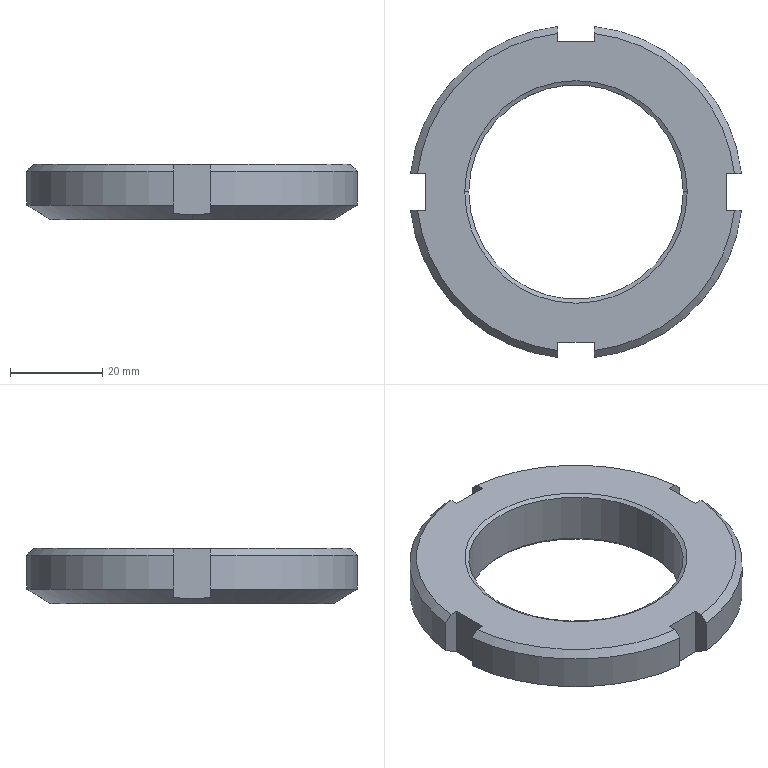Part | SolidWorks | features BaseBody 1 | 1 solid | 30 faces | box 71.554 x 71.554 x 12 mm | volume 25355 mm3 | plane 14 | cone 10 | cylinder 6 | commonest cylinder face diameters 72 x4 46.376 x2
STEP:
#1=CARTESIAN_POINT('',(-23.188,0.,-0.5));
#2=VERTEX_POINT('',#1);
#3=CARTESIAN_POINT('',(23.188,0.,-0.5));
#4=VERTEX_POINT('',#3);
#5=CARTESIAN_POINT('',(0.,0.,-0.5));
#6=DIRECTION('',(0.,0.,1.));
#7=DIRECTION('',(1.,0.,0.));
#8=AXIS2_PLACEMENT_3D('',#5,#6,#7);
#9=CIRCLE('',#8,23.188);
#10=EDGE_CURVE('',#2,#4,#9,.T.);
#11=ORIENTED_EDGE('',*,*,#10,.F.);
#12=CARTESIAN_POINT('',(-24.054,0.,0.));
#13=VERTEX_POINT('',#12);
#14=CARTESIAN_POINT('',(-24.054,0.,0.));
#15=DIRECTION('',(-0.866,0.,0.5));
#16=VECTOR('',#15,1000.);
#17=LINE('',#14,#16);
#18=EDGE_CURVE('',#2,#13,#17,.T.);
#19=ORIENTED_EDGE('',*,*,#18,.T.);
#20=CARTESIAN_POINT('',(24.054,0.,0.));
#21=VERTEX_POINT('',#20);
#22=CARTESIAN_POINT('',(0.,0.,0.));
#23=DIRECTION('',(0.,0.,-1.));
#24=DIRECTION('',(1.,0.,0.));
#25=AXIS2_PLACEMENT_3D('',#22,#23,#24);
#26=CIRCLE('',#25,24.054);
#27=EDGE_CURVE('',#21,#13,#26,.T.);
#28=ORIENTED_EDGE('',*,*,#27,.F.);
#29=CARTESIAN_POINT('',(24.054,0.,0.));
#30=DIRECTION('',(0.866,0.,0.5));
#31=VECTOR('',#30,1000.);
#32=LINE('',#29,#31);
#33=EDGE_CURVE('',#4,#21,#32,.T.);
#34=ORIENTED_EDGE('',*,*,#33,.F.);
#35=EDGE_LOOP('',(#11,#19,#28,#34));
#36=FACE_OUTER_BOUND('',#35,.T.);
#37=CARTESIAN_POINT('',(0.,0.,0.));
#38=DIRECTION('',(0.,0.,1.));
#39=DIRECTION('',(1.,0.,0.));
#40=AXIS2_PLACEMENT_3D('',#37,#38,#39);
#41=CONICAL_SURFACE('',#40,24.054,1.047);
#42=ADVANCED_FACE('',(#36),#41,.F.);
#43=CARTESIAN_POINT('',(-23.188,0.,-11.3));
#44=VERTEX_POINT('',#43);
#45=CARTESIAN_POINT('',(23.188,0.,-11.3));
#46=VERTEX_POINT('',#45);
#47=CARTESIAN_POINT('',(0.,0.,-11.3));
#48=DIRECTION('',(0.,0.,1.));
#49=DIRECTION('',(1.,0.,0.));
#50=AXIS2_PLACEMENT_3D('',#47,#48,#49);
#51=CIRCLE('',#50,23.188);
#52=EDGE_CURVE('',#44,#46,#51,.T.);
#53=ORIENTED_EDGE('',*,*,#52,.F.);
#54=CARTESIAN_POINT('',(-23.188,0.,-12.));
#55=DIRECTION('',(0.,0.,1.));
#56=VECTOR('',#55,1000.);
#57=LINE('',#54,#56);
#58=EDGE_CURVE('',#44,#2,#57,.T.);
#59=ORIENTED_EDGE('',*,*,#58,.T.);
#60=ORIENTED_EDGE('',*,*,#10,.T.);
#61=CARTESIAN_POINT('',(23.188,0.,-12.));
#62=DIRECTION('',(0.,0.,1.));
#63=VECTOR('',#62,1000.);
#64=LINE('',#61,#63);
#65=EDGE_CURVE('',#46,#4,#64,.T.);
#66=ORIENTED_EDGE('',*,*,#65,.F.);
#67=EDGE_LOOP('',(#53,#59,#60,#66));
#68=FACE_OUTER_BOUND('',#67,.T.);
#69=CARTESIAN_POINT('',(0.,0.,-12.));
#70=DIRECTION('',(0.,0.,1.));
#71=DIRECTION('',(1.,0.,0.));
#72=AXIS2_PLACEMENT_3D('',#69,#70,#71);
#73=CYLINDRICAL_SURFACE('',#72,23.188);
#74=ADVANCED_FACE('',(#68),#73,.F.);
#75=CARTESIAN_POINT('',(0.,-30.5,-12.));
#76=VERTEX_POINT('',#75);
#77=CARTESIAN_POINT('',(0.,30.5,-12.));
#78=VERTEX_POINT('',#77);
#79=CARTESIAN_POINT('',(0.,0.,-12.));
#80=DIRECTION('',(0.,0.,1.));
#81=DIRECTION('',(0.,-1.,0.));
#82=AXIS2_PLACEMENT_3D('',#79,#80,#81);
#83=CIRCLE('',#82,30.5);
#84=EDGE_CURVE('',#76,#78,#83,.T.);
#85=ORIENTED_EDGE('',*,*,#84,.T.);
#86=CARTESIAN_POINT('',(0.,32.5,-10.845));
#87=VERTEX_POINT('',#86);
#88=CARTESIAN_POINT('',(0.,36.,-8.825));
#89=DIRECTION('',(0.,0.866,0.5));
#90=VECTOR('',#89,1000.);
#91=LINE('',#88,#90);
#92=EDGE_CURVE('',#78,#87,#91,.T.);
#93=ORIENTED_EDGE('',*,*,#92,.T.);
#94=CARTESIAN_POINT('',(4.,32.5,-10.704));
#95=VERTEX_POINT('',#94);
#96=CARTESIAN_POINT('',(0.,32.5,-10.845));
#97=CARTESIAN_POINT('',(1.333,32.5,-10.845));
#98=CARTESIAN_POINT('',(2.667,32.5,-10.798));
#99=CARTESIAN_POINT('',(4.,32.5,-10.704));
#100=B_SPLINE_CURVE_WITH_KNOTS('',3,(#96,#97,#98,#99),.UNSPECIFIED.,.F.,.F.,(4,4),(0.004,0.008),.UNSPECIFIED.);
#101=EDGE_CURVE('',#87,#95,#100,.T.);
#102=ORIENTED_EDGE('',*,*,#101,.T.);
#103=CARTESIAN_POINT('',(4.,35.777,-8.825));
#104=VERTEX_POINT('',#103);
#105=CARTESIAN_POINT('',(4.,32.5,-10.704));
#106=CARTESIAN_POINT('',(4.,33.593,-10.078));
#107=CARTESIAN_POINT('',(4.,34.685,-9.451));
#108=CARTESIAN_POINT('',(4.,35.777,-8.825));
#109=B_SPLINE_CURVE_WITH_KNOTS('',3,(#105,#106,#107,#108),.UNSPECIFIED.,.F.,.F.,(4,4),(0.,0.003778),.UNSPECIFIED.);
#110=EDGE_CURVE('',#95,#104,#109,.T.);
#111=ORIENTED_EDGE('',*,*,#110,.T.);
#112=CARTESIAN_POINT('',(35.777,4.,-8.825));
#113=VERTEX_POINT('',#112);
#114=CARTESIAN_POINT('',(0.,0.,-8.825));
#115=DIRECTION('',(0.,0.,-1.));
#116=DIRECTION('',(1.,0.,0.));
#117=AXIS2_PLACEMENT_3D('',#114,#115,#116);
#118=CIRCLE('',#117,36.);
#119=EDGE_CURVE('',#104,#113,#118,.T.);
#120=ORIENTED_EDGE('',*,*,#119,.T.);
#121=CARTESIAN_POINT('',(32.5,4.,-10.704));
#122=VERTEX_POINT('',#121);
#123=CARTESIAN_POINT('',(35.777,4.,-8.825));
#124=CARTESIAN_POINT('',(34.685,4.,-9.451));
#125=CARTESIAN_POINT('',(33.593,4.,-10.078));
#126=CARTESIAN_POINT('',(32.5,4.,-10.704));
#127=B_SPLINE_CURVE_WITH_KNOTS('',3,(#123,#124,#125,#126),.UNSPECIFIED.,.F.,.F.,(4,4),(0.,0.003778),.UNSPECIFIED.);
#128=EDGE_CURVE('',#113,#122,#127,.T.);
#129=ORIENTED_EDGE('',*,*,#128,.T.);
#130=CARTESIAN_POINT('',(32.5,-4.,-10.704));
#131=VERTEX_POINT('',#130);
#132=CARTESIAN_POINT('',(32.5,4.,-10.704));
#133=CARTESIAN_POINT('',(32.5,1.337,-10.892));
#134=CARTESIAN_POINT('',(32.5,-1.337,-10.892));
#135=CARTESIAN_POINT('',(32.5,-4.,-10.704));
#136=B_SPLINE_CURVE_WITH_KNOTS('',3,(#132,#133,#134,#135),.UNSPECIFIED.,.F.,.F.,(4,4),(-0.004003,0.004003),.UNSPECIFIED.);
#137=EDGE_CURVE('',#122,#131,#136,.T.);
#138=ORIENTED_EDGE('',*,*,#137,.T.);
#139=CARTESIAN_POINT('',(35.777,-4.,-8.825));
#140=VERTEX_POINT('',#139);
#141=CARTESIAN_POINT('',(32.5,-4.,-10.704));
#142=CARTESIAN_POINT('',(33.593,-4.,-10.078));
#143=CARTESIAN_POINT('',(34.685,-4.,-9.451));
#144=CARTESIAN_POINT('',(35.777,-4.,-8.825));
#145=B_SPLINE_CURVE_WITH_KNOTS('',3,(#141,#142,#143,#144),.UNSPECIFIED.,.F.,.F.,(4,4),(0.,0.003778),.UNSPECIFIED.);
#146=EDGE_CURVE('',#131,#140,#145,.T.);
#147=ORIENTED_EDGE('',*,*,#146,.T.);
#148=CARTESIAN_POINT('',(4.,-35.777,-8.825));
#149=VERTEX_POINT('',#148);
#150=CARTESIAN_POINT('',(0.,0.,-8.825));
#151=DIRECTION('',(0.,0.,-1.));
#152=DIRECTION('',(1.,0.,0.));
#153=AXIS2_PLACEMENT_3D('',#150,#151,#152);
#154=CIRCLE('',#153,36.);
#155=EDGE_CURVE('',#140,#149,#154,.T.);
#156=ORIENTED_EDGE('',*,*,#155,.T.);
#157=CARTESIAN_POINT('',(4.,-32.5,-10.704));
#158=VERTEX_POINT('',#157);
#159=CARTESIAN_POINT('',(4.,-35.777,-8.825));
#160=CARTESIAN_POINT('',(4.,-34.685,-9.451));
#161=CARTESIAN_POINT('',(4.,-33.593,-10.078));
#162=CARTESIAN_POINT('',(4.,-32.5,-10.704));
#163=B_SPLINE_CURVE_WITH_KNOTS('',3,(#159,#160,#161,#162),.UNSPECIFIED.,.F.,.F.,(4,4),(0.,0.003778),.UNSPECIFIED.);
#164=EDGE_CURVE('',#149,#158,#163,.T.);
#165=ORIENTED_EDGE('',*,*,#164,.T.);
#166=CARTESIAN_POINT('',(0.,-32.5,-10.845));
#167=VERTEX_POINT('',#166);
#168=CARTESIAN_POINT('',(4.,-32.5,-10.704));
#169=CARTESIAN_POINT('',(2.667,-32.5,-10.798));
#170=CARTESIAN_POINT('',(1.333,-32.5,-10.845));
#171=CARTESIAN_POINT('',(0.,-32.5,-10.845));
#172=B_SPLINE_CURVE_WITH_KNOTS('',3,(#168,#169,#170,#171),.UNSPECIFIED.,.F.,.F.,(4,4),(0.,0.004),.UNSPECIFIED.);
#173=EDGE_CURVE('',#158,#167,#172,.T.);
#174=ORIENTED_EDGE('',*,*,#173,.T.);
#175=CARTESIAN_POINT('',(0.,-36.,-8.825));
#176=DIRECTION('',(0.,-0.866,0.5));
#177=VECTOR('',#176,1000.);
#178=LINE('',#175,#177);
#179=EDGE_CURVE('',#76,#167,#178,.T.);
#180=ORIENTED_EDGE('',*,*,#179,.F.);
#181=EDGE_LOOP('',(#85,#93,#102,#111,#120,#129,#138,#147,#156,#165,#174,#180));
#182=FACE_OUTER_BOUND('',#181,.T.);
#183=CARTESIAN_POINT('',(0.,0.,-8.825));
#184=DIRECTION('',(0.,0.,1.));
#185=DIRECTION('',(0.,-1.,0.));
#186=AXIS2_PLACEMENT_3D('',#183,#184,#185);
#187=CONICAL_SURFACE('',#186,36.,1.047);
#188=ADVANCED_FACE('',(#182),#187,.T.);
#189=ORIENTED_EDGE('',*,*,#52,.T.);
#190=CARTESIAN_POINT('',(23.888,0.,-12.));
#191=VERTEX_POINT('',#190);
#192=CARTESIAN_POINT('',(23.888,0.,-12.));
#193=DIRECTION('',(0.7071,0.,-0.7071));
#194=VECTOR('',#193,1000.);
#195=LINE('',#192,#194);
#196=EDGE_CURVE('',#46,#191,#195,.T.);
#197=ORIENTED_EDGE('',*,*,#196,.T.);
#198=CARTESIAN_POINT('',(-23.888,0.,-12.));
#199=VERTEX_POINT('',#198);
#200=CARTESIAN_POINT('',(0.,0.,-12.));
#201=DIRECTION('',(0.,0.,1.));
#202=DIRECTION('',(-1.,0.,0.));
#203=AXIS2_PLACEMENT_3D('',#200,#201,#202);
#204=CIRCLE('',#203,23.888);
#205=EDGE_CURVE('',#199,#191,#204,.T.);
#206=ORIENTED_EDGE('',*,*,#205,.F.);
#207=CARTESIAN_POINT('',(-23.888,0.,-12.));
#208=DIRECTION('',(-0.7071,0.,-0.7071));
#209=VECTOR('',#208,1000.);
#210=LINE('',#207,#209);
#211=EDGE_CURVE('',#44,#199,#210,.T.);
#212=ORIENTED_EDGE('',*,*,#211,.F.);
#213=EDGE_LOOP('',(#189,#197,#206,#212));
#214=FACE_OUTER_BOUND('',#213,.T.);
#215=CARTESIAN_POINT('',(0.,0.,-12.));
#216=DIRECTION('',(0.,0.,-1.));
#217=DIRECTION('',(-1.,0.,0.));
#218=AXIS2_PLACEMENT_3D('',#215,#216,#217);
#219=CONICAL_SURFACE('',#218,23.888,0.7854);
#220=ADVANCED_FACE('',(#214),#219,.F.);
#221=ORIENTED_EDGE('',*,*,#27,.T.);
#222=CARTESIAN_POINT('',(0.,0.,0.));
#223=DIRECTION('',(0.,0.,-1.));
#224=DIRECTION('',(1.,0.,0.));
#225=AXIS2_PLACEMENT_3D('',#222,#223,#224);
#226=CIRCLE('',#225,24.054);
#227=EDGE_CURVE('',#13,#21,#226,.T.);
#228=ORIENTED_EDGE('',*,*,#227,.T.);
#229=EDGE_LOOP('',(#221,#228));
#230=FACE_BOUND('',#229,.T.);
#231=CARTESIAN_POINT('',(-34.267,4.,0.));
#232=VERTEX_POINT('',#231);
#233=CARTESIAN_POINT('',(-32.5,4.,0.));
#234=VERTEX_POINT('',#233);
#235=CARTESIAN_POINT('',(0.,4.,0.));
#236=DIRECTION('',(1.,0.,0.));
#237=VECTOR('',#236,1000.);
#238=LINE('',#235,#237);
#239=EDGE_CURVE('',#232,#234,#238,.T.);
#240=ORIENTED_EDGE('',*,*,#239,.T.);
#241=CARTESIAN_POINT('',(-32.5,-4.,0.));
#242=VERTEX_POINT('',#241);
#243=CARTESIAN_POINT('',(-32.5,0.,0.));
#244=DIRECTION('',(0.,-1.,0.));
#245=VECTOR('',#244,1000.);
#246=LINE('',#243,#245);
#247=EDGE_CURVE('',#234,#242,#246,.T.);
#248=ORIENTED_EDGE('',*,*,#247,.T.);
#249=CARTESIAN_POINT('',(-34.267,-4.,0.));
#250=VERTEX_POINT('',#249);
#251=CARTESIAN_POINT('',(0.,-4.,0.));
#252=DIRECTION('',(-1.,0.,0.));
#253=VECTOR('',#252,1000.);
#254=LINE('',#251,#253);
#255=EDGE_CURVE('',#242,#250,#254,.T.);
#256=ORIENTED_EDGE('',*,*,#255,.T.);
#257=CARTESIAN_POINT('',(-4.,-34.267,0.));
#258=VERTEX_POINT('',#257);
#259=CARTESIAN_POINT('',(0.,0.,0.));
#260=DIRECTION('',(0.,0.,1.));
#261=DIRECTION('',(0.,1.,0.));
#262=AXIS2_PLACEMENT_3D('',#259,#260,#261);
#263=CIRCLE('',#262,34.5);
#264=EDGE_CURVE('',#250,#258,#263,.T.);
#265=ORIENTED_EDGE('',*,*,#264,.T.);
#266=CARTESIAN_POINT('',(-4.,-32.5,0.));
#267=VERTEX_POINT('',#266);
#268=CARTESIAN_POINT('',(-4.,0.,0.));
#269=DIRECTION('',(0.,1.,0.));
#270=VECTOR('',#269,1000.);
#271=LINE('',#268,#270);
#272=EDGE_CURVE('',#258,#267,#271,.T.);
#273=ORIENTED_EDGE('',*,*,#272,.T.);
#274=CARTESIAN_POINT('',(4.,-32.5,0.));
#275=VERTEX_POINT('',#274);
#276=CARTESIAN_POINT('',(0.,-32.5,0.));
#277=DIRECTION('',(1.,0.,0.));
#278=VECTOR('',#277,1000.);
#279=LINE('',#276,#278);
#280=EDGE_CURVE('',#267,#275,#279,.T.);
#281=ORIENTED_EDGE('',*,*,#280,.T.);
#282=CARTESIAN_POINT('',(4.,-34.267,0.));
#283=VERTEX_POINT('',#282);
#284=CARTESIAN_POINT('',(4.,0.,0.));
#285=DIRECTION('',(0.,-1.,0.));
#286=VECTOR('',#285,1000.);
#287=LINE('',#284,#286);
#288=EDGE_CURVE('',#275,#283,#287,.T.);
#289=ORIENTED_EDGE('',*,*,#288,.T.);
#290=CARTESIAN_POINT('',(34.267,-4.,0.));
#291=VERTEX_POINT('',#290);
#292=CARTESIAN_POINT('',(0.,0.,0.));
#293=DIRECTION('',(0.,0.,1.));
#294=DIRECTION('',(-1.,0.,0.));
#295=AXIS2_PLACEMENT_3D('',#292,#293,#294);
#296=CIRCLE('',#295,34.5);
#297=EDGE_CURVE('',#283,#291,#296,.T.);
#298=ORIENTED_EDGE('',*,*,#297,.T.);
#299=CARTESIAN_POINT('',(32.5,-4.,0.));
#300=VERTEX_POINT('',#299);
#301=CARTESIAN_POINT('',(0.,-4.,0.));
#302=DIRECTION('',(-1.,0.,0.));
#303=VECTOR('',#302,1000.);
#304=LINE('',#301,#303);
#305=EDGE_CURVE('',#291,#300,#304,.T.);
#306=ORIENTED_EDGE('',*,*,#305,.T.);
#307=CARTESIAN_POINT('',(32.5,4.,0.));
#308=VERTEX_POINT('',#307);
#309=CARTESIAN_POINT('',(32.5,0.,0.));
#310=DIRECTION('',(0.,1.,0.));
#311=VECTOR('',#310,1000.);
#312=LINE('',#309,#311);
#313=EDGE_CURVE('',#300,#308,#312,.T.);
#314=ORIENTED_EDGE('',*,*,#313,.T.);
#315=CARTESIAN_POINT('',(34.267,4.,0.));
#316=VERTEX_POINT('',#315);
#317=CARTESIAN_POINT('',(0.,4.,0.));
#318=DIRECTION('',(1.,0.,0.));
#319=VECTOR('',#318,1000.);
#320=LINE('',#317,#319);
#321=EDGE_CURVE('',#308,#316,#320,.T.);
#322=ORIENTED_EDGE('',*,*,#321,.T.);
#323=CARTESIAN_POINT('',(4.,34.267,0.));
#324=VERTEX_POINT('',#323);
#325=CARTESIAN_POINT('',(0.,0.,0.));
#326=DIRECTION('',(0.,0.,1.));
#327=DIRECTION('',(0.,1.,0.));
#328=AXIS2_PLACEMENT_3D('',#325,#326,#327);
#329=CIRCLE('',#328,34.5);
#330=EDGE_CURVE('',#316,#324,#329,.T.);
#331=ORIENTED_EDGE('',*,*,#330,.T.);
#332=CARTESIAN_POINT('',(4.,32.5,0.));
#333=VERTEX_POINT('',#332);
#334=CARTESIAN_POINT('',(4.,0.,0.));
#335=DIRECTION('',(0.,-1.,0.));
#336=VECTOR('',#335,1000.);
#337=LINE('',#334,#336);
#338=EDGE_CURVE('',#324,#333,#337,.T.);
#339=ORIENTED_EDGE('',*,*,#338,.T.);
#340=CARTESIAN_POINT('',(-4.,32.5,0.));
#341=VERTEX_POINT('',#340);
#342=CARTESIAN_POINT('',(0.,32.5,0.));
#343=DIRECTION('',(-1.,0.,0.));
#344=VECTOR('',#343,1000.);
#345=LINE('',#342,#344);
#346=EDGE_CURVE('',#333,#341,#345,.T.);
#347=ORIENTED_EDGE('',*,*,#346,.T.);
#348=CARTESIAN_POINT('',(-4.,34.267,0.));
#349=VERTEX_POINT('',#348);
#350=CARTESIAN_POINT('',(-4.,0.,0.));
#351=DIRECTION('',(0.,1.,0.));
#352=VECTOR('',#351,1000.);
#353=LINE('',#350,#352);
#354=EDGE_CURVE('',#341,#349,#353,.T.);
#355=ORIENTED_EDGE('',*,*,#354,.T.);
#356=CARTESIAN_POINT('',(0.,0.,0.));
#357=DIRECTION('',(0.,0.,1.));
#358=DIRECTION('',(-1.,0.,0.));
#359=AXIS2_PLACEMENT_3D('',#356,#357,#358);
#360=CIRCLE('',#359,34.5);
#361=EDGE_CURVE('',#349,#232,#360,.T.);
#362=ORIENTED_EDGE('',*,*,#361,.T.);
#363=EDGE_LOOP('',(#240,#248,#256,#265,#273,#281,#289,#298,#306,#314,#322,#331,#339,#347,#355,#362));
#364=FACE_OUTER_BOUND('',#363,.T.);
#365=CARTESIAN_POINT('',(0.,0.,0.));
#366=DIRECTION('',(0.,0.,1.));
#367=DIRECTION('',(1.,0.,0.));
#368=AXIS2_PLACEMENT_3D('',#365,#366,#367);
#369=PLANE('',#368);
#370=ADVANCED_FACE('',(#230,#364),#369,.T.);
#371=ORIENTED_EDGE('',*,*,#18,.F.);
#372=CARTESIAN_POINT('',(0.,0.,-0.5));
#373=DIRECTION('',(0.,0.,1.));
#374=DIRECTION('',(1.,0.,0.));
#375=AXIS2_PLACEMENT_3D('',#372,#373,#374);
#376=CIRCLE('',#375,23.188);
#377=EDGE_CURVE('',#4,#2,#376,.T.);
#378=ORIENTED_EDGE('',*,*,#377,.F.);
#379=ORIENTED_EDGE('',*,*,#33,.T.);
#380=ORIENTED_EDGE('',*,*,#227,.F.);
#381=EDGE_LOOP('',(#371,#378,#379,#380));
#382=FACE_OUTER_BOUND('',#381,.T.);
#383=CARTESIAN_POINT('',(0.,0.,0.));
#384=DIRECTION('',(0.,0.,1.));
#385=DIRECTION('',(1.,0.,0.));
#386=AXIS2_PLACEMENT_3D('',#383,#384,#385);
#387=CONICAL_SURFACE('',#386,24.054,1.047);
#388=ADVANCED_FACE('',(#382),#387,.F.);
#389=ORIENTED_EDGE('',*,*,#247,.F.);
#390=CARTESIAN_POINT('',(-32.5,4.,-10.704));
#391=VERTEX_POINT('',#390);
#392=CARTESIAN_POINT('',(-32.5,4.,0.));
#393=DIRECTION('',(0.,0.,1.));
#394=VECTOR('',#393,1000.);
#395=LINE('',#392,#394);
#396=EDGE_CURVE('',#391,#234,#395,.T.);
#397=ORIENTED_EDGE('',*,*,#396,.F.);
#398=CARTESIAN_POINT('',(-32.5,-4.,-10.704));
#399=VERTEX_POINT('',#398);
#400=CARTESIAN_POINT('',(-32.5,-4.,-10.704));
#401=CARTESIAN_POINT('',(-32.5,-1.337,-10.892));
#402=CARTESIAN_POINT('',(-32.5,1.337,-10.892));
#403=CARTESIAN_POINT('',(-32.5,4.,-10.704));
#404=B_SPLINE_CURVE_WITH_KNOTS('',3,(#400,#401,#402,#403),.UNSPECIFIED.,.F.,.F.,(4,4),(-0.004003,0.004003),.UNSPECIFIED.);
#405=EDGE_CURVE('',#399,#391,#404,.T.);
#406=ORIENTED_EDGE('',*,*,#405,.F.);
#407=CARTESIAN_POINT('',(-32.5,-4.,0.));
#408=DIRECTION('',(0.,0.,-1.));
#409=VECTOR('',#408,1000.);
#410=LINE('',#407,#409);
#411=EDGE_CURVE('',#242,#399,#410,.T.);
#412=ORIENTED_EDGE('',*,*,#411,.F.);
#413=EDGE_LOOP('',(#389,#397,#406,#412));
#414=FACE_OUTER_BOUND('',#413,.T.);
#415=CARTESIAN_POINT('',(-32.5,-4.,0.));
#416=DIRECTION('',(1.,0.,0.));
#417=DIRECTION('',(0.,1.,0.));
#418=AXIS2_PLACEMENT_3D('',#415,#416,#417);
#419=PLANE('',#418);
#420=ADVANCED_FACE('',(#414),#419,.F.);
#421=CARTESIAN_POINT('',(-35.777,4.,-8.825));
#422=VERTEX_POINT('',#421);
#423=CARTESIAN_POINT('',(-35.777,4.,-1.5));
#424=VERTEX_POINT('',#423);
#425=CARTESIAN_POINT('',(-35.777,4.,0.));
#426=DIRECTION('',(0.,0.,1.));
#427=VECTOR('',#426,1000.);
#428=LINE('',#425,#427);
#429=EDGE_CURVE('',#422,#424,#428,.T.);
#430=ORIENTED_EDGE('',*,*,#429,.F.);
#431=CARTESIAN_POINT('',(-32.5,4.,-10.704));
#432=CARTESIAN_POINT('',(-33.593,4.,-10.078));
#433=CARTESIAN_POINT('',(-34.685,4.,-9.451));
#434=CARTESIAN_POINT('',(-35.777,4.,-8.825));
#435=B_SPLINE_CURVE_WITH_KNOTS('',3,(#431,#432,#433,#434),.UNSPECIFIED.,.F.,.F.,(4,4),(0.,0.003778),.UNSPECIFIED.);
#436=EDGE_CURVE('',#391,#422,#435,.T.);
#437=ORIENTED_EDGE('',*,*,#436,.F.);
#438=ORIENTED_EDGE('',*,*,#396,.T.);
#439=ORIENTED_EDGE('',*,*,#239,.F.);
#440=CARTESIAN_POINT('',(-35.777,4.,-1.5));
#441=CARTESIAN_POINT('',(-35.274,4.,-0.9999));
#442=CARTESIAN_POINT('',(-34.771,4.,-0.4999));
#443=CARTESIAN_POINT('',(-34.267,4.,0.));
#444=B_SPLINE_CURVE_WITH_KNOTS('',3,(#440,#441,#442,#443),.UNSPECIFIED.,.F.,.F.,(4,4),(0.,0.002128),.UNSPECIFIED.);
#445=EDGE_CURVE('',#424,#232,#444,.T.);
#446=ORIENTED_EDGE('',*,*,#445,.F.);
#447=EDGE_LOOP('',(#430,#437,#438,#439,#446));
#448=FACE_OUTER_BOUND('',#447,.T.);
#449=CARTESIAN_POINT('',(-32.5,4.,0.));
#450=DIRECTION('',(0.,1.,0.));
#451=DIRECTION('',(-1.,0.,0.));
#452=AXIS2_PLACEMENT_3D('',#449,#450,#451);
#453=PLANE('',#452);
#454=ADVANCED_FACE('',(#448),#453,.F.);
#455=CARTESIAN_POINT('',(-4.,35.777,-1.5));
#456=VERTEX_POINT('',#455);
#457=CARTESIAN_POINT('',(-4.,34.267,0.));
#458=CARTESIAN_POINT('',(-4.,34.771,-0.4999));
#459=CARTESIAN_POINT('',(-4.,35.274,-0.9999));
#460=CARTESIAN_POINT('',(-4.,35.777,-1.5));
#461=B_SPLINE_CURVE_WITH_KNOTS('',3,(#457,#458,#459,#460),.UNSPECIFIED.,.F.,.F.,(4,4),(0.,0.002128),.UNSPECIFIED.);
#462=EDGE_CURVE('',#349,#456,#461,.T.);
#463=ORIENTED_EDGE('',*,*,#462,.T.);
#464=CARTESIAN_POINT('',(0.,0.,-1.5));
#465=DIRECTION('',(0.,0.,1.));
#466=DIRECTION('',(-1.,0.,0.));
#467=AXIS2_PLACEMENT_3D('',#464,#465,#466);
#468=CIRCLE('',#467,36.);
#469=EDGE_CURVE('',#456,#424,#468,.T.);
#470=ORIENTED_EDGE('',*,*,#469,.T.);
#471=ORIENTED_EDGE('',*,*,#445,.T.);
#472=ORIENTED_EDGE('',*,*,#361,.F.);
#473=EDGE_LOOP('',(#463,#470,#471,#472));
#474=FACE_OUTER_BOUND('',#473,.T.);
#475=CARTESIAN_POINT('',(0.,0.,-1.5));
#476=DIRECTION('',(0.,0.,-1.));
#477=DIRECTION('',(-1.,0.,0.));
#478=AXIS2_PLACEMENT_3D('',#475,#476,#477);
#479=CONICAL_SURFACE('',#478,36.,0.7854);
#480=ADVANCED_FACE('',(#474),#479,.T.);
#481=ORIENTED_EDGE('',*,*,#354,.F.);
#482=CARTESIAN_POINT('',(-4.,32.5,-10.704));
#483=VERTEX_POINT('',#482);
#484=CARTESIAN_POINT('',(-4.,32.5,0.));
#485=DIRECTION('',(0.,0.,1.));
#486=VECTOR('',#485,1000.);
#487=LINE('',#484,#486);
#488=EDGE_CURVE('',#483,#341,#487,.T.);
#489=ORIENTED_EDGE('',*,*,#488,.F.);
#490=CARTESIAN_POINT('',(-4.,35.777,-8.825));
#491=VERTEX_POINT('',#490);
#492=CARTESIAN_POINT('',(-4.,35.777,-8.825));
#493=CARTESIAN_POINT('',(-4.,34.685,-9.451));
#494=CARTESIAN_POINT('',(-4.,33.593,-10.078));
#495=CARTESIAN_POINT('',(-4.,32.5,-10.704));
#496=B_SPLINE_CURVE_WITH_KNOTS('',3,(#492,#493,#494,#495),.UNSPECIFIED.,.F.,.F.,(4,4),(0.,0.003778),.UNSPECIFIED.);
#497=EDGE_CURVE('',#491,#483,#496,.T.);
#498=ORIENTED_EDGE('',*,*,#497,.F.);
#499=CARTESIAN_POINT('',(-4.,35.777,0.));
#500=DIRECTION('',(0.,0.,-1.));
#501=VECTOR('',#500,1000.);
#502=LINE('',#499,#501);
#503=EDGE_CURVE('',#456,#491,#502,.T.);
#504=ORIENTED_EDGE('',*,*,#503,.F.);
#505=ORIENTED_EDGE('',*,*,#462,.F.);
#506=EDGE_LOOP('',(#481,#489,#498,#504,#505));
#507=FACE_OUTER_BOUND('',#506,.T.);
#508=CARTESIAN_POINT('',(-4.,35.777,0.));
#509=DIRECTION('',(-1.,0.,0.));
#510=DIRECTION('',(0.,-1.,0.));
#511=AXIS2_PLACEMENT_3D('',#508,#509,#510);
#512=PLANE('',#511);
#513=ADVANCED_FACE('',(#507),#512,.F.);
#514=ORIENTED_EDGE('',*,*,#346,.F.);
#515=CARTESIAN_POINT('',(4.,32.5,0.));
#516=DIRECTION('',(0.,0.,1.));
#517=VECTOR('',#516,1000.);
#518=LINE('',#515,#517);
#519=EDGE_CURVE('',#95,#333,#518,.T.);
#520=ORIENTED_EDGE('',*,*,#519,.F.);
#521=ORIENTED_EDGE('',*,*,#101,.F.);
#522=CARTESIAN_POINT('',(-4.,32.5,-10.704));
#523=CARTESIAN_POINT('',(-2.667,32.5,-10.798));
#524=CARTESIAN_POINT('',(-1.333,32.5,-10.845));
#525=CARTESIAN_POINT('',(0.,32.5,-10.845));
#526=B_SPLINE_CURVE_WITH_KNOTS('',3,(#522,#523,#524,#525),.UNSPECIFIED.,.F.,.F.,(4,4),(0.,0.004),.UNSPECIFIED.);
#527=EDGE_CURVE('',#483,#87,#526,.T.);
#528=ORIENTED_EDGE('',*,*,#527,.F.);
#529=ORIENTED_EDGE('',*,*,#488,.T.);
#530=EDGE_LOOP('',(#514,#520,#521,#528,#529));
#531=FACE_OUTER_BOUND('',#530,.T.);
#532=CARTESIAN_POINT('',(-4.,32.5,0.));
#533=DIRECTION('',(0.,-1.,0.));
#534=DIRECTION('',(1.,0.,0.));
#535=AXIS2_PLACEMENT_3D('',#532,#533,#534);
#536=PLANE('',#535);
#537=ADVANCED_FACE('',(#531),#536,.F.);
#538=CARTESIAN_POINT('',(4.,35.777,-1.5));
#539=VERTEX_POINT('',#538);
#540=CARTESIAN_POINT('',(4.,35.777,0.));
#541=DIRECTION('',(0.,0.,1.));
#542=VECTOR('',#541,1000.);
#543=LINE('',#540,#542);
#544=EDGE_CURVE('',#104,#539,#543,.T.);
#545=ORIENTED_EDGE('',*,*,#544,.F.);
#546=ORIENTED_EDGE('',*,*,#110,.F.);
#547=ORIENTED_EDGE('',*,*,#519,.T.);
#548=ORIENTED_EDGE('',*,*,#338,.F.);
#549=CARTESIAN_POINT('',(4.,35.777,-1.5));
#550=CARTESIAN_POINT('',(4.,35.274,-0.9999));
#551=CARTESIAN_POINT('',(4.,34.771,-0.4999));
#552=CARTESIAN_POINT('',(4.,34.267,0.));
#553=B_SPLINE_CURVE_WITH_KNOTS('',3,(#549,#550,#551,#552),.UNSPECIFIED.,.F.,.F.,(4,4),(0.,0.002128),.UNSPECIFIED.);
#554=EDGE_CURVE('',#539,#324,#553,.T.);
#555=ORIENTED_EDGE('',*,*,#554,.F.);
#556=EDGE_LOOP('',(#545,#546,#547,#548,#555));
#557=FACE_OUTER_BOUND('',#556,.T.);
#558=CARTESIAN_POINT('',(4.,32.5,0.));
#559=DIRECTION('',(1.,0.,0.));
#560=DIRECTION('',(0.,1.,0.));
#561=AXIS2_PLACEMENT_3D('',#558,#559,#560);
#562=PLANE('',#561);
#563=ADVANCED_FACE('',(#557),#562,.F.);
#564=CARTESIAN_POINT('',(35.777,4.,-1.5));
#565=VERTEX_POINT('',#564);
#566=CARTESIAN_POINT('',(34.267,4.,0.));
#567=CARTESIAN_POINT('',(34.771,4.,-0.4999));
#568=CARTESIAN_POINT('',(35.274,4.,-0.9999));
#569=CARTESIAN_POINT('',(35.777,4.,-1.5));
#570=B_SPLINE_CURVE_WITH_KNOTS('',3,(#566,#567,#568,#569),.UNSPECIFIED.,.F.,.F.,(4,4),(0.,0.002128),.UNSPECIFIED.);
#571=EDGE_CURVE('',#316,#565,#570,.T.);
#572=ORIENTED_EDGE('',*,*,#571,.T.);
#573=CARTESIAN_POINT('',(0.,0.,-1.5));
#574=DIRECTION('',(0.,0.,1.));
#575=DIRECTION('',(-1.,0.,0.));
#576=AXIS2_PLACEMENT_3D('',#573,#574,#575);
#577=CIRCLE('',#576,36.);
#578=EDGE_CURVE('',#565,#539,#577,.T.);
#579=ORIENTED_EDGE('',*,*,#578,.T.);
#580=ORIENTED_EDGE('',*,*,#554,.T.);
#581=ORIENTED_EDGE('',*,*,#330,.F.);
#582=EDGE_LOOP('',(#572,#579,#580,#581));
#583=FACE_OUTER_BOUND('',#582,.T.);
#584=CARTESIAN_POINT('',(0.,0.,-1.5));
#585=DIRECTION('',(0.,0.,-1.));
#586=DIRECTION('',(0.,1.,0.));
#587=AXIS2_PLACEMENT_3D('',#584,#585,#586);
#588=CONICAL_SURFACE('',#587,36.,0.7854);
#589=ADVANCED_FACE('',(#583),#588,.T.);
#590=ORIENTED_EDGE('',*,*,#571,.F.);
#591=ORIENTED_EDGE('',*,*,#321,.F.);
#592=CARTESIAN_POINT('',(32.5,4.,0.));
#593=DIRECTION('',(0.,0.,1.));
#594=VECTOR('',#593,1000.);
#595=LINE('',#592,#594);
#596=EDGE_CURVE('',#122,#308,#595,.T.);
#597=ORIENTED_EDGE('',*,*,#596,.F.);
#598=ORIENTED_EDGE('',*,*,#128,.F.);
#599=CARTESIAN_POINT('',(35.777,4.,0.));
#600=DIRECTION('',(0.,0.,-1.));
#601=VECTOR('',#600,1000.);
#602=LINE('',#599,#601);
#603=EDGE_CURVE('',#565,#113,#602,.T.);
#604=ORIENTED_EDGE('',*,*,#603,.F.);
#605=EDGE_LOOP('',(#590,#591,#597,#598,#604));
#606=FACE_OUTER_BOUND('',#605,.T.);
#607=CARTESIAN_POINT('',(35.777,4.,0.));
#608=DIRECTION('',(0.,1.,0.));
#609=DIRECTION('',(-1.,0.,0.));
#610=AXIS2_PLACEMENT_3D('',#607,#608,#609);
#611=PLANE('',#610);
#612=ADVANCED_FACE('',(#606),#611,.F.);
#613=ORIENTED_EDGE('',*,*,#313,.F.);
#614=CARTESIAN_POINT('',(32.5,-4.,0.));
#615=DIRECTION('',(0.,0.,1.));
#616=VECTOR('',#615,1000.);
#617=LINE('',#614,#616);
#618=EDGE_CURVE('',#131,#300,#617,.T.);
#619=ORIENTED_EDGE('',*,*,#618,.F.);
#620=ORIENTED_EDGE('',*,*,#137,.F.);
#621=ORIENTED_EDGE('',*,*,#596,.T.);
#622=EDGE_LOOP('',(#613,#619,#620,#621));
#623=FACE_OUTER_BOUND('',#622,.T.);
#624=CARTESIAN_POINT('',(32.5,4.,0.));
#625=DIRECTION('',(-1.,0.,0.));
#626=DIRECTION('',(0.,-1.,0.));
#627=AXIS2_PLACEMENT_3D('',#624,#625,#626);
#628=PLANE('',#627);
#629=ADVANCED_FACE('',(#623),#628,.F.);
#630=ORIENTED_EDGE('',*,*,#305,.F.);
#631=CARTESIAN_POINT('',(35.777,-4.,-1.5));
#632=VERTEX_POINT('',#631);
#633=CARTESIAN_POINT('',(35.777,-4.,-1.5));
#634=CARTESIAN_POINT('',(35.274,-4.,-0.9999));
#635=CARTESIAN_POINT('',(34.771,-4.,-0.4999));
#636=CARTESIAN_POINT('',(34.267,-4.,0.));
#637=B_SPLINE_CURVE_WITH_KNOTS('',3,(#633,#634,#635,#636),.UNSPECIFIED.,.F.,.F.,(4,4),(0.,0.002128),.UNSPECIFIED.);
#638=EDGE_CURVE('',#632,#291,#637,.T.);
#639=ORIENTED_EDGE('',*,*,#638,.F.);
#640=CARTESIAN_POINT('',(35.777,-4.,0.));
#641=DIRECTION('',(0.,0.,1.));
#642=VECTOR('',#641,1000.);
#643=LINE('',#640,#642);
#644=EDGE_CURVE('',#140,#632,#643,.T.);
#645=ORIENTED_EDGE('',*,*,#644,.F.);
#646=ORIENTED_EDGE('',*,*,#146,.F.);
#647=ORIENTED_EDGE('',*,*,#618,.T.);
#648=EDGE_LOOP('',(#630,#639,#645,#646,#647));
#649=FACE_OUTER_BOUND('',#648,.T.);
#650=CARTESIAN_POINT('',(32.5,-4.,0.));
#651=DIRECTION('',(0.,-1.,0.));
#652=DIRECTION('',(1.,0.,0.));
#653=AXIS2_PLACEMENT_3D('',#650,#651,#652);
#654=PLANE('',#653);
#655=ADVANCED_FACE('',(#649),#654,.F.);
#656=CARTESIAN_POINT('',(4.,-35.777,-1.5));
#657=VERTEX_POINT('',#656);
#658=CARTESIAN_POINT('',(4.,-34.267,0.));
#659=CARTESIAN_POINT('',(4.,-34.771,-0.4999));
#660=CARTESIAN_POINT('',(4.,-35.274,-0.9999));
#661=CARTESIAN_POINT('',(4.,-35.777,-1.5));
#662=B_SPLINE_CURVE_WITH_KNOTS('',3,(#658,#659,#660,#661),.UNSPECIFIED.,.F.,.F.,(4,4),(0.,0.002128),.UNSPECIFIED.);
#663=EDGE_CURVE('',#283,#657,#662,.T.);
#664=ORIENTED_EDGE('',*,*,#663,.T.);
#665=CARTESIAN_POINT('',(0.,0.,-1.5));
#666=DIRECTION('',(0.,0.,1.));
#667=DIRECTION('',(-1.,0.,0.));
#668=AXIS2_PLACEMENT_3D('',#665,#666,#667);
#669=CIRCLE('',#668,36.);
#670=EDGE_CURVE('',#657,#632,#669,.T.);
#671=ORIENTED_EDGE('',*,*,#670,.T.);
#672=ORIENTED_EDGE('',*,*,#638,.T.);
#673=ORIENTED_EDGE('',*,*,#297,.F.);
#674=EDGE_LOOP('',(#664,#671,#672,#673));
#675=FACE_OUTER_BOUND('',#674,.T.);
#676=CARTESIAN_POINT('',(0.,0.,-1.5));
#677=DIRECTION('',(0.,0.,-1.));
#678=DIRECTION('',(-1.,0.,0.));
#679=AXIS2_PLACEMENT_3D('',#676,#677,#678);
#680=CONICAL_SURFACE('',#679,36.,0.7854);
#681=ADVANCED_FACE('',(#675),#680,.T.);
#682=ORIENTED_EDGE('',*,*,#663,.F.);
#683=ORIENTED_EDGE('',*,*,#288,.F.);
#684=CARTESIAN_POINT('',(4.,-32.5,0.));
#685=DIRECTION('',(0.,0.,1.));
#686=VECTOR('',#685,1000.);
#687=LINE('',#684,#686);
#688=EDGE_CURVE('',#158,#275,#687,.T.);
#689=ORIENTED_EDGE('',*,*,#688,.F.);
#690=ORIENTED_EDGE('',*,*,#164,.F.);
#691=CARTESIAN_POINT('',(4.,-35.777,0.));
#692=DIRECTION('',(0.,0.,-1.));
#693=VECTOR('',#692,1000.);
#694=LINE('',#691,#693);
#695=EDGE_CURVE('',#657,#149,#694,.T.);
#696=ORIENTED_EDGE('',*,*,#695,.F.);
#697=EDGE_LOOP('',(#682,#683,#689,#690,#696));
#698=FACE_OUTER_BOUND('',#697,.T.);
#699=CARTESIAN_POINT('',(4.,-35.777,0.));
#700=DIRECTION('',(1.,0.,0.));
#701=DIRECTION('',(0.,0.,-1.));
#702=AXIS2_PLACEMENT_3D('',#699,#700,#701);
#703=PLANE('',#702);
#704=ADVANCED_FACE('',(#698),#703,.F.);
#705=ORIENTED_EDGE('',*,*,#280,.F.);
#706=CARTESIAN_POINT('',(-4.,-32.5,-10.704));
#707=VERTEX_POINT('',#706);
#708=CARTESIAN_POINT('',(-4.,-32.5,0.));
#709=DIRECTION('',(0.,0.,1.));
#710=VECTOR('',#709,1000.);
#711=LINE('',#708,#710);
#712=EDGE_CURVE('',#707,#267,#711,.T.);
#713=ORIENTED_EDGE('',*,*,#712,.F.);
#714=CARTESIAN_POINT('',(0.,-32.5,-10.845));
#715=CARTESIAN_POINT('',(-1.333,-32.5,-10.845));
#716=CARTESIAN_POINT('',(-2.667,-32.5,-10.798));
#717=CARTESIAN_POINT('',(-4.,-32.5,-10.704));
#718=B_SPLINE_CURVE_WITH_KNOTS('',3,(#714,#715,#716,#717),.UNSPECIFIED.,.F.,.F.,(4,4),(0.004,0.008),.UNSPECIFIED.);
#719=EDGE_CURVE('',#167,#707,#718,.T.);
#720=ORIENTED_EDGE('',*,*,#719,.F.);
#721=ORIENTED_EDGE('',*,*,#173,.F.);
#722=ORIENTED_EDGE('',*,*,#688,.T.);
#723=EDGE_LOOP('',(#705,#713,#720,#721,#722));
#724=FACE_OUTER_BOUND('',#723,.T.);
#725=CARTESIAN_POINT('',(4.,-32.5,0.));
#726=DIRECTION('',(0.,1.,0.));
#727=DIRECTION('',(0.,0.,1.));
#728=AXIS2_PLACEMENT_3D('',#725,#726,#727);
#729=PLANE('',#728);
#730=ADVANCED_FACE('',(#724),#729,.F.);
#731=ORIENTED_EDGE('',*,*,#272,.F.);
#732=CARTESIAN_POINT('',(-4.,-35.777,-1.5));
#733=VERTEX_POINT('',#732);
#734=CARTESIAN_POINT('',(-4.,-35.777,-1.5));
#735=CARTESIAN_POINT('',(-4.,-35.274,-0.9999));
#736=CARTESIAN_POINT('',(-4.,-34.771,-0.4999));
#737=CARTESIAN_POINT('',(-4.,-34.267,0.));
#738=B_SPLINE_CURVE_WITH_KNOTS('',3,(#734,#735,#736,#737),.UNSPECIFIED.,.F.,.F.,(4,4),(0.,0.002128),.UNSPECIFIED.);
#739=EDGE_CURVE('',#733,#258,#738,.T.);
#740=ORIENTED_EDGE('',*,*,#739,.F.);
#741=CARTESIAN_POINT('',(-4.,-35.777,-8.825));
#742=VERTEX_POINT('',#741);
#743=CARTESIAN_POINT('',(-4.,-35.777,0.));
#744=DIRECTION('',(0.,0.,1.));
#745=VECTOR('',#744,1000.);
#746=LINE('',#743,#745);
#747=EDGE_CURVE('',#742,#733,#746,.T.);
#748=ORIENTED_EDGE('',*,*,#747,.F.);
#749=CARTESIAN_POINT('',(-4.,-32.5,-10.704));
#750=CARTESIAN_POINT('',(-4.,-33.593,-10.078));
#751=CARTESIAN_POINT('',(-4.,-34.685,-9.451));
#752=CARTESIAN_POINT('',(-4.,-35.777,-8.825));
#753=B_SPLINE_CURVE_WITH_KNOTS('',3,(#749,#750,#751,#752),.UNSPECIFIED.,.F.,.F.,(4,4),(0.,0.003778),.UNSPECIFIED.);
#754=EDGE_CURVE('',#707,#742,#753,.T.);
#755=ORIENTED_EDGE('',*,*,#754,.F.);
#756=ORIENTED_EDGE('',*,*,#712,.T.);
#757=EDGE_LOOP('',(#731,#740,#748,#755,#756));
#758=FACE_OUTER_BOUND('',#757,.T.);
#759=CARTESIAN_POINT('',(-4.,-32.5,0.));
#760=DIRECTION('',(-1.,0.,0.));
#761=DIRECTION('',(0.,-1.,0.));
#762=AXIS2_PLACEMENT_3D('',#759,#760,#761);
#763=PLANE('',#762);
#764=ADVANCED_FACE('',(#758),#763,.F.);
#765=ORIENTED_EDGE('',*,*,#739,.T.);
#766=ORIENTED_EDGE('',*,*,#264,.F.);
#767=CARTESIAN_POINT('',(-35.777,-4.,-1.5));
#768=VERTEX_POINT('',#767);
#769=CARTESIAN_POINT('',(-34.267,-4.,0.));
#770=CARTESIAN_POINT('',(-34.771,-4.,-0.4999));
#771=CARTESIAN_POINT('',(-35.274,-4.,-0.9999));
#772=CARTESIAN_POINT('',(-35.777,-4.,-1.5));
#773=B_SPLINE_CURVE_WITH_KNOTS('',3,(#769,#770,#771,#772),.UNSPECIFIED.,.F.,.F.,(4,4),(0.,0.002128),.UNSPECIFIED.);
#774=EDGE_CURVE('',#250,#768,#773,.T.);
#775=ORIENTED_EDGE('',*,*,#774,.T.);
#776=CARTESIAN_POINT('',(0.,0.,-1.5));
#777=DIRECTION('',(0.,0.,1.));
#778=DIRECTION('',(-1.,0.,0.));
#779=AXIS2_PLACEMENT_3D('',#776,#777,#778);
#780=CIRCLE('',#779,36.);
#781=EDGE_CURVE('',#768,#733,#780,.T.);
#782=ORIENTED_EDGE('',*,*,#781,.T.);
#783=EDGE_LOOP('',(#765,#766,#775,#782));
#784=FACE_OUTER_BOUND('',#783,.T.);
#785=CARTESIAN_POINT('',(0.,0.,-1.5));
#786=DIRECTION('',(0.,0.,-1.));
#787=DIRECTION('',(0.,1.,0.));
#788=AXIS2_PLACEMENT_3D('',#785,#786,#787);
#789=CONICAL_SURFACE('',#788,36.,0.7854);
#790=ADVANCED_FACE('',(#784),#789,.T.);
#791=ORIENTED_EDGE('',*,*,#255,.F.);
#792=ORIENTED_EDGE('',*,*,#411,.T.);
#793=CARTESIAN_POINT('',(-35.777,-4.,-8.825));
#794=VERTEX_POINT('',#793);
#795=CARTESIAN_POINT('',(-35.777,-4.,-8.825));
#796=CARTESIAN_POINT('',(-34.685,-4.,-9.451));
#797=CARTESIAN_POINT('',(-33.593,-4.,-10.078));
#798=CARTESIAN_POINT('',(-32.5,-4.,-10.704));
#799=B_SPLINE_CURVE_WITH_KNOTS('',3,(#795,#796,#797,#798),.UNSPECIFIED.,.F.,.F.,(4,4),(0.,0.003778),.UNSPECIFIED.);
#800=EDGE_CURVE('',#794,#399,#799,.T.);
#801=ORIENTED_EDGE('',*,*,#800,.F.);
#802=CARTESIAN_POINT('',(-35.777,-4.,0.));
#803=DIRECTION('',(0.,0.,-1.));
#804=VECTOR('',#803,1000.);
#805=LINE('',#802,#804);
#806=EDGE_CURVE('',#768,#794,#805,.T.);
#807=ORIENTED_EDGE('',*,*,#806,.F.);
#808=ORIENTED_EDGE('',*,*,#774,.F.);
#809=EDGE_LOOP('',(#791,#792,#801,#807,#808));
#810=FACE_OUTER_BOUND('',#809,.T.);
#811=CARTESIAN_POINT('',(-35.777,-4.,0.));
#812=DIRECTION('',(0.,-1.,0.));
#813=DIRECTION('',(1.,0.,0.));
#814=AXIS2_PLACEMENT_3D('',#811,#812,#813);
#815=PLANE('',#814);
#816=ADVANCED_FACE('',(#810),#815,.F.);
#817=ORIENTED_EDGE('',*,*,#58,.F.);
#818=CARTESIAN_POINT('',(0.,0.,-11.3));
#819=DIRECTION('',(0.,0.,1.));
#820=DIRECTION('',(1.,0.,0.));
#821=AXIS2_PLACEMENT_3D('',#818,#819,#820);
#822=CIRCLE('',#821,23.188);
#823=EDGE_CURVE('',#46,#44,#822,.T.);
#824=ORIENTED_EDGE('',*,*,#823,.F.);
#825=ORIENTED_EDGE('',*,*,#65,.T.);
#826=ORIENTED_EDGE('',*,*,#377,.T.);
#827=EDGE_LOOP('',(#817,#824,#825,#826));
#828=FACE_OUTER_BOUND('',#827,.T.);
#829=CARTESIAN_POINT('',(0.,0.,-12.));
#830=DIRECTION('',(0.,0.,1.));
#831=DIRECTION('',(1.,0.,0.));
#832=AXIS2_PLACEMENT_3D('',#829,#830,#831);
#833=CYLINDRICAL_SURFACE('',#832,23.188);
#834=ADVANCED_FACE('',(#828),#833,.F.);
#835=ORIENTED_EDGE('',*,*,#92,.F.);
#836=CARTESIAN_POINT('',(0.,0.,-12.));
#837=DIRECTION('',(0.,0.,1.));
#838=DIRECTION('',(0.,-1.,0.));
#839=AXIS2_PLACEMENT_3D('',#836,#837,#838);
#840=CIRCLE('',#839,30.5);
#841=EDGE_CURVE('',#78,#76,#840,.T.);
#842=ORIENTED_EDGE('',*,*,#841,.T.);
#843=ORIENTED_EDGE('',*,*,#179,.T.);
#844=ORIENTED_EDGE('',*,*,#719,.T.);
#845=ORIENTED_EDGE('',*,*,#754,.T.);
#846=CARTESIAN_POINT('',(0.,0.,-8.825));
#847=DIRECTION('',(0.,0.,-1.));
#848=DIRECTION('',(1.,0.,0.));
#849=AXIS2_PLACEMENT_3D('',#846,#847,#848);
#850=CIRCLE('',#849,36.);
#851=EDGE_CURVE('',#742,#794,#850,.T.);
#852=ORIENTED_EDGE('',*,*,#851,.T.);
#853=ORIENTED_EDGE('',*,*,#800,.T.);
#854=ORIENTED_EDGE('',*,*,#405,.T.);
#855=ORIENTED_EDGE('',*,*,#436,.T.);
#856=CARTESIAN_POINT('',(0.,0.,-8.825));
#857=DIRECTION('',(0.,0.,-1.));
#858=DIRECTION('',(1.,0.,0.));
#859=AXIS2_PLACEMENT_3D('',#856,#857,#858);
#860=CIRCLE('',#859,36.);
#861=EDGE_CURVE('',#422,#491,#860,.T.);
#862=ORIENTED_EDGE('',*,*,#861,.T.);
#863=ORIENTED_EDGE('',*,*,#497,.T.);
#864=ORIENTED_EDGE('',*,*,#527,.T.);
#865=EDGE_LOOP('',(#835,#842,#843,#844,#845,#852,#853,#854,#855,#862,#863,#864));
#866=FACE_OUTER_BOUND('',#865,.T.);
#867=CARTESIAN_POINT('',(0.,0.,-8.825));
#868=DIRECTION('',(0.,0.,1.));
#869=DIRECTION('',(0.,-1.,0.));
#870=AXIS2_PLACEMENT_3D('',#867,#868,#869);
#871=CONICAL_SURFACE('',#870,36.,1.047);
#872=ADVANCED_FACE('',(#866),#871,.T.);
#873=ORIENTED_EDGE('',*,*,#503,.T.);
#874=ORIENTED_EDGE('',*,*,#861,.F.);
#875=ORIENTED_EDGE('',*,*,#429,.T.);
#876=ORIENTED_EDGE('',*,*,#469,.F.);
#877=EDGE_LOOP('',(#873,#874,#875,#876));
#878=FACE_OUTER_BOUND('',#877,.T.);
#879=CARTESIAN_POINT('',(0.,0.,-12.));
#880=DIRECTION('',(0.,0.,1.));
#881=DIRECTION('',(1.,0.,0.));
#882=AXIS2_PLACEMENT_3D('',#879,#880,#881);
#883=CYLINDRICAL_SURFACE('',#882,36.);
#884=ADVANCED_FACE('',(#878),#883,.T.);
#885=ORIENTED_EDGE('',*,*,#603,.T.);
#886=ORIENTED_EDGE('',*,*,#119,.F.);
#887=ORIENTED_EDGE('',*,*,#544,.T.);
#888=ORIENTED_EDGE('',*,*,#578,.F.);
#889=EDGE_LOOP('',(#885,#886,#887,#888));
#890=FACE_OUTER_BOUND('',#889,.T.);
#891=CARTESIAN_POINT('',(0.,0.,-12.));
#892=DIRECTION('',(0.,0.,1.));
#893=DIRECTION('',(1.,0.,0.));
#894=AXIS2_PLACEMENT_3D('',#891,#892,#893);
#895=CYLINDRICAL_SURFACE('',#894,36.);
#896=ADVANCED_FACE('',(#890),#895,.T.);
#897=ORIENTED_EDGE('',*,*,#695,.T.);
#898=ORIENTED_EDGE('',*,*,#155,.F.);
#899=ORIENTED_EDGE('',*,*,#644,.T.);
#900=ORIENTED_EDGE('',*,*,#670,.F.);
#901=EDGE_LOOP('',(#897,#898,#899,#900));
#902=FACE_OUTER_BOUND('',#901,.T.);
#903=CARTESIAN_POINT('',(0.,0.,-12.));
#904=DIRECTION('',(0.,0.,1.));
#905=DIRECTION('',(1.,0.,0.));
#906=AXIS2_PLACEMENT_3D('',#903,#904,#905);
#907=CYLINDRICAL_SURFACE('',#906,36.);
#908=ADVANCED_FACE('',(#902),#907,.T.);
#909=ORIENTED_EDGE('',*,*,#747,.T.);
#910=ORIENTED_EDGE('',*,*,#781,.F.);
#911=ORIENTED_EDGE('',*,*,#806,.T.);
#912=ORIENTED_EDGE('',*,*,#851,.F.);
#913=EDGE_LOOP('',(#909,#910,#911,#912));
#914=FACE_OUTER_BOUND('',#913,.T.);
#915=CARTESIAN_POINT('',(0.,0.,-12.));
#916=DIRECTION('',(0.,0.,1.));
#917=DIRECTION('',(1.,0.,0.));
#918=AXIS2_PLACEMENT_3D('',#915,#916,#917);
#919=CYLINDRICAL_SURFACE('',#918,36.);
#920=ADVANCED_FACE('',(#914),#919,.T.);
#921=ORIENTED_EDGE('',*,*,#196,.F.);
#922=ORIENTED_EDGE('',*,*,#823,.T.);
#923=ORIENTED_EDGE('',*,*,#211,.T.);
#924=CARTESIAN_POINT('',(0.,0.,-12.));
#925=DIRECTION('',(0.,0.,1.));
#926=DIRECTION('',(-1.,0.,0.));
#927=AXIS2_PLACEMENT_3D('',#924,#925,#926);
#928=CIRCLE('',#927,23.888);
#929=EDGE_CURVE('',#191,#199,#928,.T.);
#930=ORIENTED_EDGE('',*,*,#929,.F.);
#931=EDGE_LOOP('',(#921,#922,#923,#930));
#932=FACE_OUTER_BOUND('',#931,.T.);
#933=CARTESIAN_POINT('',(0.,0.,-12.));
#934=DIRECTION('',(0.,0.,-1.));
#935=DIRECTION('',(-1.,0.,0.));
#936=AXIS2_PLACEMENT_3D('',#933,#934,#935);
#937=CONICAL_SURFACE('',#936,23.888,0.7854);
#938=ADVANCED_FACE('',(#932),#937,.F.);
#939=ORIENTED_EDGE('',*,*,#84,.F.);
#940=ORIENTED_EDGE('',*,*,#841,.F.);
#941=EDGE_LOOP('',(#939,#940));
#942=FACE_OUTER_BOUND('',#941,.T.);
#943=ORIENTED_EDGE('',*,*,#205,.T.);
#944=ORIENTED_EDGE('',*,*,#929,.T.);
#945=EDGE_LOOP('',(#943,#944));
#946=FACE_BOUND('',#945,.T.);
#947=CARTESIAN_POINT('',(0.,0.,-12.));
#948=DIRECTION('',(0.,0.,1.));
#949=DIRECTION('',(1.,0.,0.));
#950=AXIS2_PLACEMENT_3D('',#947,#948,#949);
#951=PLANE('',#950);
#952=ADVANCED_FACE('',(#942,#946),#951,.F.);
#953=CLOSED_SHELL('',(#42,#74,#188,#220,#370,#388,#420,#454,#480,#513,#537,#563,#589,#612,#629,#655,#681,#704,#730,#764,#790,#816,#834,#872,#884,#896,#908,#920,#938,#952));
#954=MANIFOLD_SOLID_BREP('',#953);
#955=CARTESIAN_POINT('',(0.,0.,0.));
#956=DIRECTION('',(0.,0.,1.));
#957=DIRECTION('',(1.,0.,0.));
#958=AXIS2_PLACEMENT_3D('',#955,#956,#957);
#959=(LENGTH_UNIT()NAMED_UNIT(*)SI_UNIT(.MILLI.,.METRE.));
#960=UNCERTAINTY_MEASURE_WITH_UNIT(LENGTH_MEASURE(0.00001),#959,'','');
#961=(NAMED_UNIT(*)PLANE_ANGLE_UNIT()SI_UNIT($,.RADIAN.));
#962=(NAMED_UNIT(*)SI_UNIT($,.STERADIAN.)SOLID_ANGLE_UNIT());
#963=(GEOMETRIC_REPRESENTATION_CONTEXT(3)GLOBAL_UNCERTAINTY_ASSIGNED_CONTEXT((#960))GLOBAL_UNIT_ASSIGNED_CONTEXT((#959,#961,#962))REPRESENTATION_CONTEXT('',''));
#964=ADVANCED_BREP_SHAPE_REPRESENTATION('',(#954,#958),#963);